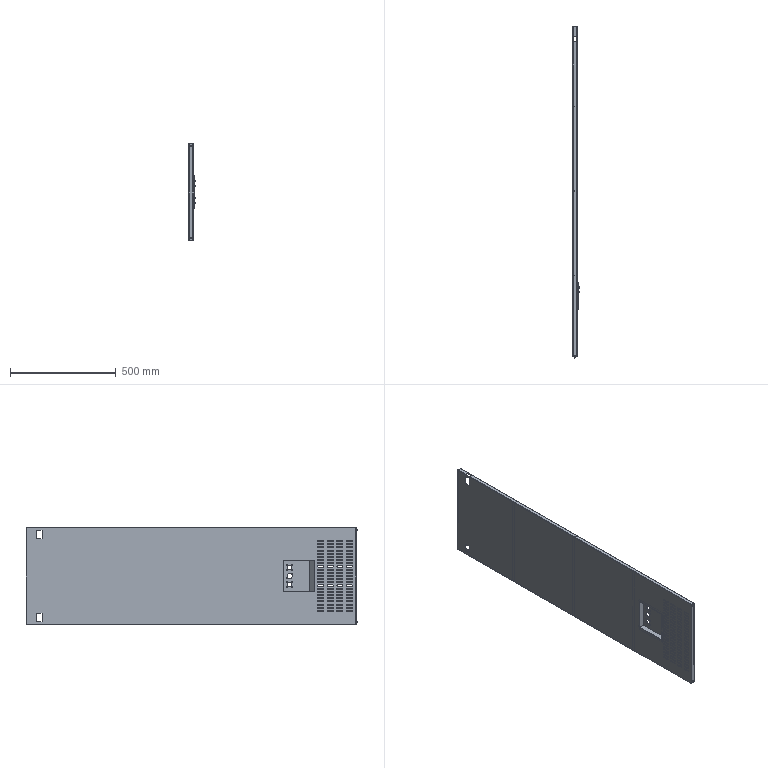Part | SolidWorks | features CompositeCurve 3, LocalLPattern 1, ReferencePattern 1 | 10 solids | 721 faces | box 30 x 1568 x 458 mm | volume 871583 mm3 | plane 382 | cylinder 304 | spline 19 | torus 16 | commonest cylinder face diameters 5 x184 0.2 x20 3.5 x20 4.5 x20 2.2 x18 7.5 x16